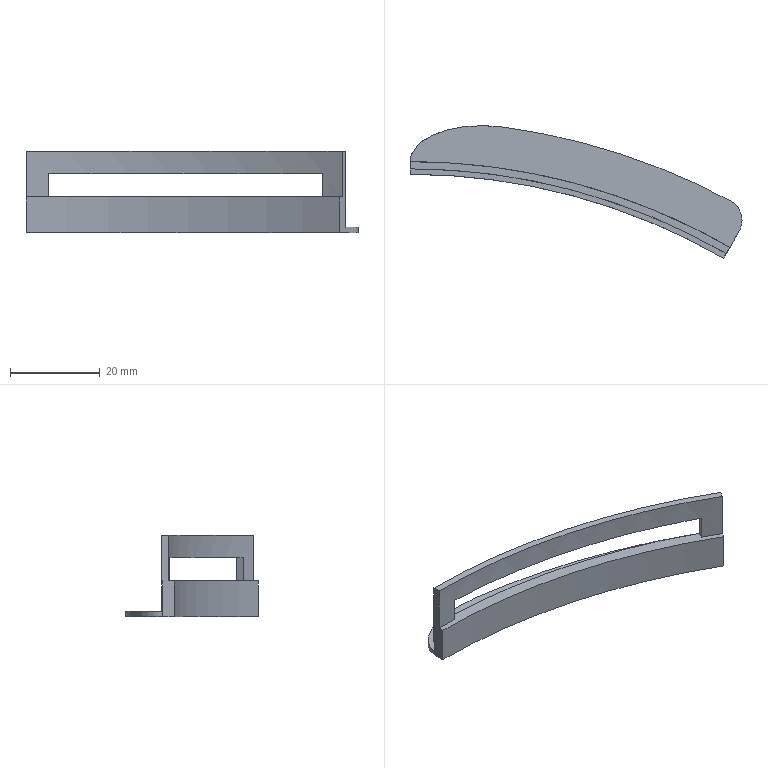Part | SolidWorks | features BaseBody 1 | 1 solid | 16 faces | box 74.127 x 29.637 x 18.2 mm | volume 3120 mm3 | plane 8 | cylinder 6 | cone 1 | spline 1 | commonest cylinder face diameters 10 x2 280 x1 282.4 x1 285.6 x1 304 x1
STEP:
#1=CARTESIAN_POINT('',(74.127,129.732,0.0213));
#2=VERTEX_POINT('',#1);
#3=CARTESIAN_POINT('',(73.457,127.232,0.01564));
#4=VERTEX_POINT('',#3);
#5=CARTESIAN_POINT('',(74.127,129.732,0.0213));
#6=CARTESIAN_POINT('',(74.127,129.293,0.02044));
#7=CARTESIAN_POINT('',(74.07,128.863,0.01953));
#8=CARTESIAN_POINT('',(73.902,128.232,0.0181));
#9=CARTESIAN_POINT('',(73.831,128.023,0.01762));
#10=CARTESIAN_POINT('',(73.664,127.619,0.01663));
#11=CARTESIAN_POINT('',(73.567,127.422,0.01614));
#12=CARTESIAN_POINT('',(73.457,127.232,0.01564));
#13=B_SPLINE_CURVE_WITH_KNOTS('',3,(#5,#6,#7,#8,#9,#10,#11,#12),.UNSPECIFIED.,.F.,.F.,(4,2,2,4),(0.,0.0013,0.00195,0.002599),.UNSPECIFIED.);
#14=EDGE_CURVE('',#2,#4,#13,.T.);
#15=ORIENTED_EDGE('',*,*,#14,.F.);
#16=CARTESIAN_POINT('',(74.127,129.732,1.2));
#17=VERTEX_POINT('',#16);
#18=CARTESIAN_POINT('',(74.127,129.732,0.008536));
#19=DIRECTION('',(0.,0.,1.));
#20=VECTOR('',#19,1000.);
#21=LINE('',#18,#20);
#22=EDGE_CURVE('',#2,#17,#21,.T.);
#23=ORIENTED_EDGE('',*,*,#22,.T.);
#24=CARTESIAN_POINT('',(73.457,127.232,1.2));
#25=VERTEX_POINT('',#24);
#26=CARTESIAN_POINT('',(69.127,129.732,1.2));
#27=DIRECTION('',(0.,0.,1.));
#28=DIRECTION('',(1.,0.,0.));
#29=AXIS2_PLACEMENT_3D('',#26,#27,#28);
#30=CIRCLE('',#29,5.);
#31=EDGE_CURVE('',#25,#17,#30,.T.);
#32=ORIENTED_EDGE('',*,*,#31,.F.);
#33=CARTESIAN_POINT('',(73.457,127.232,9.1));
#34=DIRECTION('',(0.,0.,-1.));
#35=VECTOR('',#34,1000.);
#36=LINE('',#33,#35);
#37=EDGE_CURVE('',#25,#4,#36,.T.);
#38=ORIENTED_EDGE('',*,*,#37,.T.);
#39=EDGE_LOOP('',(#15,#23,#32,#38));
#40=FACE_OUTER_BOUND('',#39,.T.);
#41=CARTESIAN_POINT('',(69.127,129.732,0.008536));
#42=DIRECTION('',(0.,0.,1.));
#43=DIRECTION('',(1.,0.,0.));
#44=AXIS2_PLACEMENT_3D('',#41,#42,#43);
#45=CYLINDRICAL_SURFACE('',#44,5.);
#46=ADVANCED_FACE('',(#40),#45,.T.);
#47=ORIENTED_EDGE('',*,*,#22,.F.);
#48=CARTESIAN_POINT('',(71.479,134.145,0.02715));
#49=VERTEX_POINT('',#48);
#50=CARTESIAN_POINT('',(71.479,134.145,0.02715));
#51=CARTESIAN_POINT('',(71.88,133.931,0.02715));
#52=CARTESIAN_POINT('',(72.243,133.668,0.02701));
#53=CARTESIAN_POINT('',(72.733,133.203,0.02662));
#54=CARTESIAN_POINT('',(72.888,133.035,0.02645));
#55=CARTESIAN_POINT('',(73.17,132.684,0.02606));
#56=CARTESIAN_POINT('',(73.298,132.5,0.02584));
#57=CARTESIAN_POINT('',(73.644,131.923,0.02508));
#58=CARTESIAN_POINT('',(73.826,131.501,0.02445));
#59=CARTESIAN_POINT('',(74.005,130.853,0.02337));
#60=CARTESIAN_POINT('',(74.051,130.633,0.02299));
#61=CARTESIAN_POINT('',(74.112,130.187,0.02218));
#62=CARTESIAN_POINT('',(74.127,129.959,0.02175));
#63=CARTESIAN_POINT('',(74.127,129.732,0.0213));
#64=B_SPLINE_CURVE_WITH_KNOTS('',3,(#50,#51,#52,#53,#54,#55,#56,#57,#58,#59,#60,#61,#62,#63),.UNSPECIFIED.,.F.,.F.,(4,2,2,2,2,2,4),(-0.005377,-0.004033,-0.003361,-0.002689,-0.001344,-0.0006722,0.),.UNSPECIFIED.);
#65=EDGE_CURVE('',#49,#2,#64,.T.);
#66=ORIENTED_EDGE('',*,*,#65,.F.);
#67=CARTESIAN_POINT('',(71.479,134.145,1.2));
#68=VERTEX_POINT('',#67);
#69=CARTESIAN_POINT('',(71.479,134.145,0.6136));
#70=DIRECTION('',(0.,0.,1.));
#71=VECTOR('',#70,1000.);
#72=LINE('',#69,#71);
#73=EDGE_CURVE('',#49,#68,#72,.T.);
#74=ORIENTED_EDGE('',*,*,#73,.T.);
#75=CARTESIAN_POINT('',(69.127,129.732,1.2));
#76=DIRECTION('',(0.,0.,1.));
#77=DIRECTION('',(1.,0.,0.));
#78=AXIS2_PLACEMENT_3D('',#75,#76,#77);
#79=CIRCLE('',#78,5.);
#80=EDGE_CURVE('',#17,#68,#79,.T.);
#81=ORIENTED_EDGE('',*,*,#80,.F.);
#82=EDGE_LOOP('',(#47,#66,#74,#81));
#83=FACE_OUTER_BOUND('',#82,.T.);
#84=CARTESIAN_POINT('',(69.127,129.732,0.008536));
#85=DIRECTION('',(0.,0.,1.));
#86=DIRECTION('',(1.,0.,0.));
#87=AXIS2_PLACEMENT_3D('',#84,#85,#86);
#88=CYLINDRICAL_SURFACE('',#87,5.);
#89=ADVANCED_FACE('',(#83),#88,.T.);
#90=CARTESIAN_POINT('',(21.111,150.527,0.02715));
#91=VERTEX_POINT('',#90);
#92=CARTESIAN_POINT('',(-0.000000007,142.604,0.005891));
#93=VERTEX_POINT('',#92);
#94=CARTESIAN_POINT('',(21.111,150.527,0.02715));
#95=CARTESIAN_POINT('',(19.061,150.814,0.02715));
#96=CARTESIAN_POINT('',(17.016,150.927,0.02685));
#97=CARTESIAN_POINT('',(13.958,150.832,0.02595));
#98=CARTESIAN_POINT('',(12.94,150.755,0.02558));
#99=CARTESIAN_POINT('',(11.416,150.562,0.02487));
#100=CARTESIAN_POINT('',(10.908,150.485,0.02461));
#101=CARTESIAN_POINT('',(9.894,150.302,0.02404));
#102=CARTESIAN_POINT('',(9.385,150.195,0.02372));
#103=CARTESIAN_POINT('',(7.872,149.828,0.02269));
#104=CARTESIAN_POINT('',(6.886,149.522,0.02189));
#105=CARTESIAN_POINT('',(5.452,148.942,0.02045));
#106=CARTESIAN_POINT('',(4.982,148.728,0.01993));
#107=CARTESIAN_POINT('',(4.06,148.247,0.01878));
#108=CARTESIAN_POINT('',(3.61,147.981,0.01815));
#109=CARTESIAN_POINT('',(2.755,147.394,0.01678));
#110=CARTESIAN_POINT('',(2.348,147.073,0.01604));
#111=CARTESIAN_POINT('',(1.589,146.353,0.01439));
#112=CARTESIAN_POINT('',(1.247,145.963,0.0135));
#113=CARTESIAN_POINT('',(0.8075,145.322,0.01204));
#114=CARTESIAN_POINT('',(0.6729,145.097,0.01153));
#115=CARTESIAN_POINT('',(0.4361,144.63,0.01048));
#116=CARTESIAN_POINT('',(0.3351,144.391,0.009933));
#117=CARTESIAN_POINT('',(0.08855,143.653,0.008264));
#118=CARTESIAN_POINT('',(0.,143.13,0.007081));
#119=CARTESIAN_POINT('',(-0.000000007,142.604,0.005891));
#120=B_SPLINE_CURVE_WITH_KNOTS('',3,(#94,#95,#96,#97,#98,#99,#100,#101,#102,#103,#104,#105,#106,#107,#108,#109,#110,#111,#112,#113,#114,#115,#116,#117,#118,#119),.UNSPECIFIED.,.F.,.F.,(4,2,2,2,2,2,2,2,2,2,2,2,4),(0.,0.006119,0.009179,0.01071,0.01224,0.0153,0.01683,0.01836,0.01989,0.02142,0.02218,0.02295,0.02448),.UNSPECIFIED.);
#121=EDGE_CURVE('',#91,#93,#120,.T.);
#122=ORIENTED_EDGE('',*,*,#121,.F.);
#123=CARTESIAN_POINT('',(0.,0.,0.02715));
#124=DIRECTION('',(0.,0.,1.));
#125=DIRECTION('',(1.,0.,0.));
#126=AXIS2_PLACEMENT_3D('',#123,#124,#125);
#127=CIRCLE('',#126,152.);
#128=EDGE_CURVE('',#49,#91,#127,.T.);
#129=ORIENTED_EDGE('',*,*,#128,.F.);
#130=ORIENTED_EDGE('',*,*,#65,.T.);
#131=ORIENTED_EDGE('',*,*,#14,.T.);
#132=CARTESIAN_POINT('',(70.,121.244,0.));
#133=VERTEX_POINT('',#132);
#134=CARTESIAN_POINT('',(73.,126.44,0.01357));
#135=DIRECTION('',(0.5,0.866,0.002262));
#136=VECTOR('',#135,1000.);
#137=LINE('',#134,#136);
#138=EDGE_CURVE('',#133,#4,#137,.T.);
#139=ORIENTED_EDGE('',*,*,#138,.F.);
#140=CARTESIAN_POINT('',(-0.000000014,140.,0.));
#141=VERTEX_POINT('',#140);
#142=CARTESIAN_POINT('',(0.,0.,0.));
#143=DIRECTION('',(0.,0.,-1.));
#144=DIRECTION('',(1.,0.,0.));
#145=AXIS2_PLACEMENT_3D('',#142,#143,#144);
#146=CIRCLE('',#145,140.);
#147=EDGE_CURVE('',#141,#133,#146,.T.);
#148=ORIENTED_EDGE('',*,*,#147,.F.);
#149=CARTESIAN_POINT('',(-0.00000003,146.,0.01357));
#150=DIRECTION('',(0.,-1.,-0.002262));
#151=VECTOR('',#150,1000.);
#152=LINE('',#149,#151);
#153=EDGE_CURVE('',#93,#141,#152,.T.);
#154=ORIENTED_EDGE('',*,*,#153,.F.);
#155=EDGE_LOOP('',(#122,#129,#130,#131,#139,#148,#154));
#156=FACE_OUTER_BOUND('',#155,.T.);
#157=CARTESIAN_POINT('',(0.,0.,0.));
#158=DIRECTION('',(0.,0.,1.));
#159=DIRECTION('',(1.,0.,0.));
#160=AXIS2_PLACEMENT_3D('',#157,#158,#159);
#161=CONICAL_SURFACE('',#160,140.,1.569);
#162=ADVANCED_FACE('',(#156),#161,.T.);
#163=ORIENTED_EDGE('',*,*,#31,.T.);
#164=ORIENTED_EDGE('',*,*,#80,.T.);
#165=CARTESIAN_POINT('',(21.111,150.527,1.2));
#166=VERTEX_POINT('',#165);
#167=CARTESIAN_POINT('',(0.,0.,1.2));
#168=DIRECTION('',(0.,0.,1.));
#169=DIRECTION('',(0.,-1.,0.));
#170=AXIS2_PLACEMENT_3D('',#167,#168,#169);
#171=CIRCLE('',#170,152.);
#172=EDGE_CURVE('',#68,#166,#171,.T.);
#173=ORIENTED_EDGE('',*,*,#172,.T.);
#174=CARTESIAN_POINT('',(0.003973,142.8,1.2));
#175=VERTEX_POINT('',#174);
#176=CARTESIAN_POINT('',(21.111,150.527,1.2));
#177=CARTESIAN_POINT('',(0.4362,153.426,1.2));
#178=CARTESIAN_POINT('',(0.003973,142.8,1.2));
#179=(BOUNDED_CURVE()B_SPLINE_CURVE(2,(#176,#177,#178),.UNSPECIFIED.,.F.,.F.)B_SPLINE_CURVE_WITH_KNOTS((3,3),(0.,0.02429),.UNSPECIFIED.)CURVE()GEOMETRIC_REPRESENTATION_ITEM()RATIONAL_B_SPLINE_CURVE((1.,0.6609,0.9907))REPRESENTATION_ITEM(''));
#180=EDGE_CURVE('',#166,#175,#179,.T.);
#181=ORIENTED_EDGE('',*,*,#180,.T.);
#182=CARTESIAN_POINT('',(71.4,123.668,1.2));
#183=VERTEX_POINT('',#182);
#184=CARTESIAN_POINT('',(0.,0.,1.2));
#185=DIRECTION('',(0.,0.,-1.));
#186=DIRECTION('',(1.,0.,0.));
#187=AXIS2_PLACEMENT_3D('',#184,#185,#186);
#188=CIRCLE('',#187,142.8);
#189=EDGE_CURVE('',#175,#183,#188,.T.);
#190=ORIENTED_EDGE('',*,*,#189,.T.);
#191=CARTESIAN_POINT('',(71.4,123.668,1.2));
#192=DIRECTION('',(0.5,0.866,0.));
#193=VECTOR('',#192,1000.);
#194=LINE('',#191,#193);
#195=EDGE_CURVE('',#183,#25,#194,.T.);
#196=ORIENTED_EDGE('',*,*,#195,.T.);
#197=EDGE_LOOP('',(#163,#164,#173,#181,#190,#196));
#198=FACE_OUTER_BOUND('',#197,.T.);
#199=CARTESIAN_POINT('',(-0.4408,123.505,1.2));
#200=DIRECTION('',(0.,0.,1.));
#201=DIRECTION('',(1.,0.,0.));
#202=AXIS2_PLACEMENT_3D('',#199,#200,#201);
#203=PLANE('',#202);
#204=ADVANCED_FACE('',(#198),#203,.T.);
#205=CARTESIAN_POINT('',(0.,141.2,18.2));
#206=VERTEX_POINT('',#205);
#207=CARTESIAN_POINT('',(0.,141.2,8.));
#208=VERTEX_POINT('',#207);
#209=CARTESIAN_POINT('',(0.,141.2,9.045));
#210=DIRECTION('',(0.,0.,-1.));
#211=VECTOR('',#210,1000.);
#212=LINE('',#209,#211);
#213=EDGE_CURVE('',#206,#208,#212,.T.);
#214=ORIENTED_EDGE('',*,*,#213,.F.);
#215=CARTESIAN_POINT('',(0.,142.8,18.2));
#216=VERTEX_POINT('',#215);
#217=CARTESIAN_POINT('',(0.,132.541,18.2));
#218=DIRECTION('',(0.,1.,0.));
#219=VECTOR('',#218,1000.);
#220=LINE('',#217,#219);
#221=EDGE_CURVE('',#206,#216,#220,.T.);
#222=ORIENTED_EDGE('',*,*,#221,.T.);
#223=CARTESIAN_POINT('',(0.001987,142.8,8.));
#224=VERTEX_POINT('',#223);
#225=CARTESIAN_POINT('',(0.,142.8,9.045));
#226=DIRECTION('',(0.,0.,1.));
#227=VECTOR('',#226,1000.);
#228=LINE('',#225,#227);
#229=EDGE_CURVE('',#224,#216,#228,.T.);
#230=ORIENTED_EDGE('',*,*,#229,.F.);
#231=CARTESIAN_POINT('',(0.,142.604,8.));
#232=VERTEX_POINT('',#231);
#233=CARTESIAN_POINT('',(0.,142.604,8.));
#234=CARTESIAN_POINT('',(0.,142.702,8.));
#235=CARTESIAN_POINT('',(0.001987,142.8,8.));
#236=(BOUNDED_CURVE()B_SPLINE_CURVE(2,(#233,#234,#235),.UNSPECIFIED.,.F.,.F.)B_SPLINE_CURVE_WITH_KNOTS((3,3),(0.,1.),.UNSPECIFIED.)CURVE()GEOMETRIC_REPRESENTATION_ITEM()RATIONAL_B_SPLINE_CURVE((1.,0.9953,0.9907))REPRESENTATION_ITEM(''));
#237=EDGE_CURVE('',#232,#224,#236,.T.);
#238=ORIENTED_EDGE('',*,*,#237,.F.);
#239=CARTESIAN_POINT('',(0.,142.604,9.045));
#240=DIRECTION('',(0.,0.,1.));
#241=VECTOR('',#240,1000.);
#242=LINE('',#239,#241);
#243=EDGE_CURVE('',#93,#232,#242,.T.);
#244=ORIENTED_EDGE('',*,*,#243,.F.);
#245=ORIENTED_EDGE('',*,*,#153,.T.);
#246=CARTESIAN_POINT('',(0.,140.,8.));
#247=VERTEX_POINT('',#246);
#248=CARTESIAN_POINT('',(0.,140.,9.045));
#249=DIRECTION('',(0.,0.,-1.));
#250=VECTOR('',#249,1000.);
#251=LINE('',#248,#250);
#252=EDGE_CURVE('',#247,#141,#251,.T.);
#253=ORIENTED_EDGE('',*,*,#252,.F.);
#254=CARTESIAN_POINT('',(0.,131.978,8.));
#255=DIRECTION('',(0.,-1.,0.));
#256=VECTOR('',#255,1000.);
#257=LINE('',#254,#256);
#258=EDGE_CURVE('',#208,#247,#257,.T.);
#259=ORIENTED_EDGE('',*,*,#258,.F.);
#260=EDGE_LOOP('',(#214,#222,#230,#238,#244,#245,#253,#259));
#261=FACE_OUTER_BOUND('',#260,.T.);
#262=CARTESIAN_POINT('',(0.,140.,-0.1092));
#263=DIRECTION('',(1.,0.,0.));
#264=DIRECTION('',(0.,1.,0.));
#265=AXIS2_PLACEMENT_3D('',#262,#263,#264);
#266=PLANE('',#265);
#267=ADVANCED_FACE('',(#261),#266,.F.);
#268=ORIENTED_EDGE('',*,*,#237,.T.);
#269=CARTESIAN_POINT('',(0.003973,142.8,8.));
#270=DIRECTION('',(0.,0.,-1.));
#271=VECTOR('',#270,1000.);
#272=LINE('',#269,#271);
#273=EDGE_CURVE('',#224,#175,#272,.T.);
#274=ORIENTED_EDGE('',*,*,#273,.T.);
#275=ORIENTED_EDGE('',*,*,#180,.F.);
#276=CARTESIAN_POINT('',(21.111,150.527,3.979));
#277=DIRECTION('',(0.,0.,-1.));
#278=VECTOR('',#277,1000.);
#279=LINE('',#276,#278);
#280=EDGE_CURVE('',#166,#91,#279,.T.);
#281=ORIENTED_EDGE('',*,*,#280,.T.);
#282=ORIENTED_EDGE('',*,*,#121,.T.);
#283=ORIENTED_EDGE('',*,*,#243,.T.);
#284=EDGE_LOOP('',(#268,#274,#275,#281,#282,#283));
#285=FACE_OUTER_BOUND('',#284,.T.);
#286=CARTESIAN_POINT('',(21.111,150.527,-0.04207));
#287=CARTESIAN_POINT('',(21.111,150.527,2.639));
#288=CARTESIAN_POINT('',(21.111,150.527,5.319));
#289=CARTESIAN_POINT('',(21.111,150.527,8.));
#290=CARTESIAN_POINT('',(0.,153.488,-0.04207));
#291=CARTESIAN_POINT('',(0.,153.488,2.639));
#292=CARTESIAN_POINT('',(0.,153.488,5.319));
#293=CARTESIAN_POINT('',(0.,153.488,8.));
#294=CARTESIAN_POINT('',(0.,142.604,-0.04207));
#295=CARTESIAN_POINT('',(0.,142.604,2.639));
#296=CARTESIAN_POINT('',(0.,142.604,5.319));
#297=CARTESIAN_POINT('',(0.,142.604,8.));
#298=(BOUNDED_SURFACE()B_SPLINE_SURFACE(2,3,((#286,#287,#288,#289),(#290,#291,#292,#293),(#294,#295,#296,#297)),.UNSPECIFIED.,.F.,.F.,.T.)B_SPLINE_SURFACE_WITH_KNOTS((3,3),(4,4),(0.,1.),(-0.00004207,0.008),.UNSPECIFIED.)GEOMETRIC_REPRESENTATION_ITEM()RATIONAL_B_SPLINE_SURFACE(((1.,1.,1.,1.),(0.6562,0.6562,0.6562,0.6562),(1.,1.,1.,1.)))REPRESENTATION_ITEM('')SURFACE());
#299=ADVANCED_FACE('',(#285),#298,.T.);
#300=ORIENTED_EDGE('',*,*,#280,.F.);
#301=ORIENTED_EDGE('',*,*,#172,.F.);
#302=ORIENTED_EDGE('',*,*,#73,.F.);
#303=ORIENTED_EDGE('',*,*,#128,.T.);
#304=EDGE_LOOP('',(#300,#301,#302,#303));
#305=FACE_OUTER_BOUND('',#304,.T.);
#306=CARTESIAN_POINT('',(0.,0.,0.02715));
#307=DIRECTION('',(0.,0.,1.));
#308=DIRECTION('',(0.,-1.,0.));
#309=AXIS2_PLACEMENT_3D('',#306,#307,#308);
#310=CYLINDRICAL_SURFACE('',#309,152.);
#311=ADVANCED_FACE('',(#305),#310,.T.);
#312=ORIENTED_EDGE('',*,*,#37,.F.);
#313=ORIENTED_EDGE('',*,*,#195,.F.);
#314=CARTESIAN_POINT('',(71.4,123.668,18.2));
#315=VERTEX_POINT('',#314);
#316=CARTESIAN_POINT('',(71.4,123.668,9.1));
#317=DIRECTION('',(0.,0.,-1.));
#318=VECTOR('',#317,1000.);
#319=LINE('',#316,#318);
#320=EDGE_CURVE('',#315,#183,#319,.T.);
#321=ORIENTED_EDGE('',*,*,#320,.F.);
#322=CARTESIAN_POINT('',(70.6,122.283,18.2));
#323=VERTEX_POINT('',#322);
#324=CARTESIAN_POINT('',(73.457,127.232,18.2));
#325=DIRECTION('',(-0.5,-0.866,0.));
#326=VECTOR('',#325,1000.);
#327=LINE('',#324,#326);
#328=EDGE_CURVE('',#315,#323,#327,.T.);
#329=ORIENTED_EDGE('',*,*,#328,.T.);
#330=CARTESIAN_POINT('',(70.6,122.283,8.));
#331=VERTEX_POINT('',#330);
#332=CARTESIAN_POINT('',(70.6,122.283,9.1));
#333=DIRECTION('',(0.,0.,1.));
#334=VECTOR('',#333,1000.);
#335=LINE('',#332,#334);
#336=EDGE_CURVE('',#331,#323,#335,.T.);
#337=ORIENTED_EDGE('',*,*,#336,.F.);
#338=CARTESIAN_POINT('',(70.,121.244,8.));
#339=VERTEX_POINT('',#338);
#340=CARTESIAN_POINT('',(70.,121.244,8.));
#341=DIRECTION('',(0.5,0.866,0.));
#342=VECTOR('',#341,1000.);
#343=LINE('',#340,#342);
#344=EDGE_CURVE('',#339,#331,#343,.T.);
#345=ORIENTED_EDGE('',*,*,#344,.F.);
#346=CARTESIAN_POINT('',(70.,121.244,9.1));
#347=DIRECTION('',(0.,0.,1.));
#348=VECTOR('',#347,1000.);
#349=LINE('',#346,#348);
#350=EDGE_CURVE('',#133,#339,#349,.T.);
#351=ORIENTED_EDGE('',*,*,#350,.F.);
#352=ORIENTED_EDGE('',*,*,#138,.T.);
#353=EDGE_LOOP('',(#312,#313,#321,#329,#337,#345,#351,#352));
#354=FACE_OUTER_BOUND('',#353,.T.);
#355=CARTESIAN_POINT('',(73.457,127.232,0.));
#356=DIRECTION('',(-0.866,0.5,0.));
#357=DIRECTION('',(-0.5,-0.866,0.));
#358=AXIS2_PLACEMENT_3D('',#355,#356,#357);
#359=PLANE('',#358);
#360=ADVANCED_FACE('',(#354),#359,.F.);
#361=ORIENTED_EDGE('',*,*,#252,.T.);
#362=ORIENTED_EDGE('',*,*,#147,.T.);
#363=ORIENTED_EDGE('',*,*,#350,.T.);
#364=CARTESIAN_POINT('',(0.,0.,8.));
#365=DIRECTION('',(0.,0.,1.));
#366=DIRECTION('',(1.,0.,0.));
#367=AXIS2_PLACEMENT_3D('',#364,#365,#366);
#368=CIRCLE('',#367,140.);
#369=EDGE_CURVE('',#339,#247,#368,.T.);
#370=ORIENTED_EDGE('',*,*,#369,.T.);
#371=EDGE_LOOP('',(#361,#362,#363,#370));
#372=FACE_OUTER_BOUND('',#371,.T.);
#373=CARTESIAN_POINT('',(0.,0.,0.));
#374=DIRECTION('',(0.,0.,1.));
#375=DIRECTION('',(1.,0.,0.));
#376=AXIS2_PLACEMENT_3D('',#373,#374,#375);
#377=CYLINDRICAL_SURFACE('',#376,140.);
#378=ADVANCED_FACE('',(#372),#377,.F.);
#379=ORIENTED_EDGE('',*,*,#273,.F.);
#380=ORIENTED_EDGE('',*,*,#229,.T.);
#381=CARTESIAN_POINT('',(0.,0.,18.2));
#382=DIRECTION('',(0.,0.,1.));
#383=DIRECTION('',(1.,0.,0.));
#384=AXIS2_PLACEMENT_3D('',#381,#382,#383);
#385=CIRCLE('',#384,142.8);
#386=EDGE_CURVE('',#315,#216,#385,.T.);
#387=ORIENTED_EDGE('',*,*,#386,.F.);
#388=ORIENTED_EDGE('',*,*,#320,.T.);
#389=ORIENTED_EDGE('',*,*,#189,.F.);
#390=EDGE_LOOP('',(#379,#380,#387,#388,#389));
#391=FACE_OUTER_BOUND('',#390,.T.);
#392=CARTESIAN_POINT('',(4.984,142.713,8.));
#393=VERTEX_POINT('',#392);
#394=CARTESIAN_POINT('',(4.984,142.713,13.2));
#395=VERTEX_POINT('',#394);
#396=CARTESIAN_POINT('',(4.984,142.713,9.7));
#397=DIRECTION('',(0.,0.,1.));
#398=VECTOR('',#397,1000.);
#399=LINE('',#396,#398);
#400=EDGE_CURVE('',#393,#395,#399,.T.);
#401=ORIENTED_EDGE('',*,*,#400,.F.);
#402=CARTESIAN_POINT('',(67.041,126.085,8.));
#403=VERTEX_POINT('',#402);
#404=CARTESIAN_POINT('',(0.,0.,8.));
#405=DIRECTION('',(0.,0.,1.));
#406=DIRECTION('',(1.,0.,0.));
#407=AXIS2_PLACEMENT_3D('',#404,#405,#406);
#408=CIRCLE('',#407,142.8);
#409=EDGE_CURVE('',#403,#393,#408,.T.);
#410=ORIENTED_EDGE('',*,*,#409,.F.);
#411=CARTESIAN_POINT('',(67.041,126.085,13.2));
#412=VERTEX_POINT('',#411);
#413=CARTESIAN_POINT('',(67.041,126.085,9.7));
#414=DIRECTION('',(0.,0.,-1.));
#415=VECTOR('',#414,1000.);
#416=LINE('',#413,#415);
#417=EDGE_CURVE('',#412,#403,#416,.T.);
#418=ORIENTED_EDGE('',*,*,#417,.F.);
#419=CARTESIAN_POINT('',(0.,0.,13.2));
#420=DIRECTION('',(0.,0.,-1.));
#421=DIRECTION('',(1.,0.,0.));
#422=AXIS2_PLACEMENT_3D('',#419,#420,#421);
#423=CIRCLE('',#422,142.8);
#424=EDGE_CURVE('',#395,#412,#423,.T.);
#425=ORIENTED_EDGE('',*,*,#424,.F.);
#426=EDGE_LOOP('',(#401,#410,#418,#425));
#427=FACE_BOUND('',#426,.T.);
#428=CARTESIAN_POINT('',(0.,0.,1.2));
#429=DIRECTION('',(0.,0.,1.));
#430=DIRECTION('',(1.,0.,0.));
#431=AXIS2_PLACEMENT_3D('',#428,#429,#430);
#432=CYLINDRICAL_SURFACE('',#431,142.8);
#433=ADVANCED_FACE('',(#391,#427),#432,.T.);
#434=CARTESIAN_POINT('',(4.928,141.114,8.));
#435=VERTEX_POINT('',#434);
#436=CARTESIAN_POINT('',(0.,0.,8.));
#437=DIRECTION('',(0.,0.,-1.));
#438=DIRECTION('',(1.,0.,0.));
#439=AXIS2_PLACEMENT_3D('',#436,#437,#438);
#440=CIRCLE('',#439,141.2);
#441=EDGE_CURVE('',#208,#435,#440,.T.);
#442=ORIENTED_EDGE('',*,*,#441,.T.);
#443=CARTESIAN_POINT('',(4.928,141.114,13.2));
#444=VERTEX_POINT('',#443);
#445=CARTESIAN_POINT('',(4.928,141.114,13.1));
#446=DIRECTION('',(0.,0.,1.));
#447=VECTOR('',#446,1000.);
#448=LINE('',#445,#447);
#449=EDGE_CURVE('',#435,#444,#448,.T.);
#450=ORIENTED_EDGE('',*,*,#449,.T.);
#451=CARTESIAN_POINT('',(66.289,124.672,13.2));
#452=VERTEX_POINT('',#451);
#453=CARTESIAN_POINT('',(0.,0.,13.2));
#454=DIRECTION('',(0.,0.,-1.));
#455=DIRECTION('',(1.,0.,0.));
#456=AXIS2_PLACEMENT_3D('',#453,#454,#455);
#457=CIRCLE('',#456,141.2);
#458=EDGE_CURVE('',#444,#452,#457,.T.);
#459=ORIENTED_EDGE('',*,*,#458,.T.);
#460=CARTESIAN_POINT('',(66.289,124.672,8.));
#461=VERTEX_POINT('',#460);
#462=CARTESIAN_POINT('',(66.289,124.672,13.1));
#463=DIRECTION('',(0.,0.,-1.));
#464=VECTOR('',#463,1000.);
#465=LINE('',#462,#464);
#466=EDGE_CURVE('',#452,#461,#465,.T.);
#467=ORIENTED_EDGE('',*,*,#466,.T.);
#468=CARTESIAN_POINT('',(0.,0.,8.));
#469=DIRECTION('',(0.,0.,-1.));
#470=DIRECTION('',(1.,0.,0.));
#471=AXIS2_PLACEMENT_3D('',#468,#469,#470);
#472=CIRCLE('',#471,141.2);
#473=EDGE_CURVE('',#461,#331,#472,.T.);
#474=ORIENTED_EDGE('',*,*,#473,.T.);
#475=ORIENTED_EDGE('',*,*,#336,.T.);
#476=CARTESIAN_POINT('',(0.,0.,18.2));
#477=DIRECTION('',(0.,0.,1.));
#478=DIRECTION('',(1.,0.,0.));
#479=AXIS2_PLACEMENT_3D('',#476,#477,#478);
#480=CIRCLE('',#479,141.2);
#481=EDGE_CURVE('',#323,#206,#480,.T.);
#482=ORIENTED_EDGE('',*,*,#481,.T.);
#483=ORIENTED_EDGE('',*,*,#213,.T.);
#484=EDGE_LOOP('',(#442,#450,#459,#467,#474,#475,#482,#483));
#485=FACE_OUTER_BOUND('',#484,.T.);
#486=CARTESIAN_POINT('',(0.,0.,8.));
#487=DIRECTION('',(0.,0.,1.));
#488=DIRECTION('',(1.,0.,0.));
#489=AXIS2_PLACEMENT_3D('',#486,#487,#488);
#490=CYLINDRICAL_SURFACE('',#489,141.2);
#491=ADVANCED_FACE('',(#485),#490,.F.);
#492=CARTESIAN_POINT('',(66.289,124.672,8.));
#493=DIRECTION('',(0.4695,0.8829,0.));
#494=VECTOR('',#493,1000.);
#495=LINE('',#492,#494);
#496=EDGE_CURVE('',#461,#403,#495,.T.);
#497=ORIENTED_EDGE('',*,*,#496,.T.);
#498=ORIENTED_EDGE('',*,*,#409,.T.);
#499=CARTESIAN_POINT('',(4.984,142.713,8.));
#500=DIRECTION('',(-0.0349,-0.9994,0.));
#501=VECTOR('',#500,1000.);
#502=LINE('',#499,#501);
#503=EDGE_CURVE('',#393,#435,#502,.T.);
#504=ORIENTED_EDGE('',*,*,#503,.T.);
#505=ORIENTED_EDGE('',*,*,#441,.F.);
#506=ORIENTED_EDGE('',*,*,#258,.T.);
#507=ORIENTED_EDGE('',*,*,#369,.F.);
#508=ORIENTED_EDGE('',*,*,#344,.T.);
#509=ORIENTED_EDGE('',*,*,#473,.F.);
#510=EDGE_LOOP('',(#497,#498,#504,#505,#506,#507,#508,#509));
#511=FACE_OUTER_BOUND('',#510,.T.);
#512=CARTESIAN_POINT('',(0.,121.115,8.));
#513=DIRECTION('',(0.,0.,1.));
#514=DIRECTION('',(1.,0.,0.));
#515=AXIS2_PLACEMENT_3D('',#512,#513,#514);
#516=PLANE('',#515);
#517=ADVANCED_FACE('',(#511),#516,.T.);
#518=ORIENTED_EDGE('',*,*,#328,.F.);
#519=ORIENTED_EDGE('',*,*,#386,.T.);
#520=ORIENTED_EDGE('',*,*,#221,.F.);
#521=ORIENTED_EDGE('',*,*,#481,.F.);
#522=EDGE_LOOP('',(#518,#519,#520,#521));
#523=FACE_OUTER_BOUND('',#522,.T.);
#524=CARTESIAN_POINT('',(71.828,122.16,18.2));
#525=DIRECTION('',(0.,0.,-1.));
#526=DIRECTION('',(-1.,0.,0.));
#527=AXIS2_PLACEMENT_3D('',#524,#525,#526);
#528=PLANE('',#527);
#529=ADVANCED_FACE('',(#523),#528,.F.);
#530=CARTESIAN_POINT('',(67.041,126.085,13.2));
#531=DIRECTION('',(-0.4695,-0.8829,0.));
#532=VECTOR('',#531,1000.);
#533=LINE('',#530,#532);
#534=EDGE_CURVE('',#412,#452,#533,.T.);
#535=ORIENTED_EDGE('',*,*,#534,.T.);
#536=ORIENTED_EDGE('',*,*,#458,.F.);
#537=CARTESIAN_POINT('',(4.928,141.114,13.2));
#538=DIRECTION('',(0.0349,0.9994,0.));
#539=VECTOR('',#538,1000.);
#540=LINE('',#537,#539);
#541=EDGE_CURVE('',#444,#395,#540,.T.);
#542=ORIENTED_EDGE('',*,*,#541,.T.);
#543=ORIENTED_EDGE('',*,*,#424,.T.);
#544=EDGE_LOOP('',(#535,#536,#542,#543));
#545=FACE_OUTER_BOUND('',#544,.T.);
#546=CARTESIAN_POINT('',(67.413,124.564,13.2));
#547=DIRECTION('',(0.,0.,-1.));
#548=DIRECTION('',(-1.,0.,0.));
#549=AXIS2_PLACEMENT_3D('',#546,#547,#548);
#550=PLANE('',#549);
#551=ADVANCED_FACE('',(#545),#550,.T.);
#552=ORIENTED_EDGE('',*,*,#503,.F.);
#553=ORIENTED_EDGE('',*,*,#400,.T.);
#554=ORIENTED_EDGE('',*,*,#541,.F.);
#555=ORIENTED_EDGE('',*,*,#449,.F.);
#556=EDGE_LOOP('',(#552,#553,#554,#555));
#557=FACE_OUTER_BOUND('',#556,.T.);
#558=CARTESIAN_POINT('',(4.928,141.114,13.2));
#559=DIRECTION('',(0.9994,-0.0349,0.));
#560=DIRECTION('',(0.,0.,-1.));
#561=AXIS2_PLACEMENT_3D('',#558,#559,#560);
#562=PLANE('',#561);
#563=ADVANCED_FACE('',(#557),#562,.T.);
#564=ORIENTED_EDGE('',*,*,#496,.F.);
#565=ORIENTED_EDGE('',*,*,#466,.F.);
#566=ORIENTED_EDGE('',*,*,#534,.F.);
#567=ORIENTED_EDGE('',*,*,#417,.T.);
#568=EDGE_LOOP('',(#564,#565,#566,#567));
#569=FACE_OUTER_BOUND('',#568,.T.);
#570=CARTESIAN_POINT('',(66.289,124.672,13.2));
#571=DIRECTION('',(0.8829,-0.4695,0.));
#572=DIRECTION('',(0.,0.,-1.));
#573=AXIS2_PLACEMENT_3D('',#570,#571,#572);
#574=PLANE('',#573);
#575=ADVANCED_FACE('',(#569),#574,.F.);
#576=CLOSED_SHELL('',(#46,#89,#162,#204,#267,#299,#311,#360,#378,#433,#491,#517,#529,#551,#563,#575));
#577=MANIFOLD_SOLID_BREP('',#576);
#578=CARTESIAN_POINT('',(0.,0.,0.));
#579=DIRECTION('',(0.,0.,1.));
#580=DIRECTION('',(1.,0.,0.));
#581=AXIS2_PLACEMENT_3D('',#578,#579,#580);
#582=(LENGTH_UNIT()NAMED_UNIT(*)SI_UNIT(.MILLI.,.METRE.));
#583=UNCERTAINTY_MEASURE_WITH_UNIT(LENGTH_MEASURE(0.00001),#582,'','');
#584=(NAMED_UNIT(*)PLANE_ANGLE_UNIT()SI_UNIT($,.RADIAN.));
#585=(NAMED_UNIT(*)SI_UNIT($,.STERADIAN.)SOLID_ANGLE_UNIT());
#586=(GEOMETRIC_REPRESENTATION_CONTEXT(3)GLOBAL_UNCERTAINTY_ASSIGNED_CONTEXT((#583))GLOBAL_UNIT_ASSIGNED_CONTEXT((#582,#584,#585))REPRESENTATION_CONTEXT('',''));
#587=ADVANCED_BREP_SHAPE_REPRESENTATION('',(#577,#581),#586);